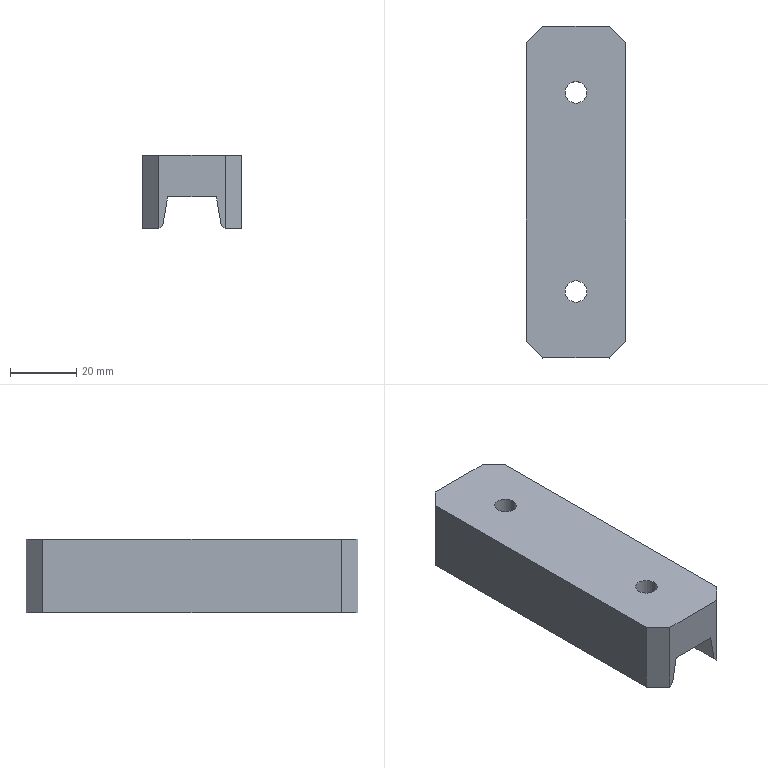Part | Creo | 1 solid | 26 faces | box 30 x 100 x 22 mm | volume 47874 mm3 | plane 18 | cylinder 8 | commonest cylinder face diameters 6.5 x4 10 x4
STEP:
#1=CARTESIAN_POINT('',(-254.325,130.,9.5));
#2=VERTEX_POINT('',#1);
#3=CARTESIAN_POINT('',(-255.826,130.,0.9848));
#4=VERTEX_POINT('',#3);
#5=CARTESIAN_POINT('',(-254.325,130.,9.5));
#6=DIRECTION('',(-0.1736,0.,-0.9848));
#7=VECTOR('',#6,8.647);
#8=LINE('',#5,#7);
#9=EDGE_CURVE('',#2,#4,#8,.T.);
#10=ORIENTED_EDGE('',*,*,#9,.F.);
#11=CARTESIAN_POINT('',(-239.675,130.,9.5));
#12=VERTEX_POINT('',#11);
#13=CARTESIAN_POINT('',(-254.325,130.,9.5));
#14=DIRECTION('',(1.,0.,0.));
#15=VECTOR('',#14,14.65);
#16=LINE('',#13,#15);
#17=EDGE_CURVE('',#2,#12,#16,.T.);
#18=ORIENTED_EDGE('',*,*,#17,.T.);
#19=CARTESIAN_POINT('',(-238.174,130.,0.9848));
#20=VERTEX_POINT('',#19);
#21=CARTESIAN_POINT('',(-238.174,130.,0.9848));
#22=DIRECTION('',(-0.1736,0.,0.9848));
#23=VECTOR('',#22,8.647);
#24=LINE('',#21,#23);
#25=EDGE_CURVE('',#20,#12,#24,.T.);
#26=ORIENTED_EDGE('',*,*,#25,.F.);
#27=CARTESIAN_POINT('',(-237.,130.,0.));
#28=VERTEX_POINT('',#27);
#29=CARTESIAN_POINT('',(-237.,130.,0.));
#30=DIRECTION('',(-0.766,0.,0.6428));
#31=VECTOR('',#30,1.532);
#32=LINE('',#29,#31);
#33=EDGE_CURVE('',#28,#20,#32,.T.);
#34=ORIENTED_EDGE('',*,*,#33,.F.);
#35=CARTESIAN_POINT('',(-237.,130.,22.));
#36=VERTEX_POINT('',#35);
#37=CARTESIAN_POINT('',(-237.,130.,0.));
#38=DIRECTION('',(0.,0.,1.));
#39=VECTOR('',#38,22.);
#40=LINE('',#37,#39);
#41=EDGE_CURVE('',#28,#36,#40,.T.);
#42=ORIENTED_EDGE('',*,*,#41,.T.);
#43=CARTESIAN_POINT('',(-257.,130.,22.));
#44=VERTEX_POINT('',#43);
#45=CARTESIAN_POINT('',(-237.,130.,22.));
#46=DIRECTION('',(-1.,0.,0.));
#47=VECTOR('',#46,20.);
#48=LINE('',#45,#47);
#49=EDGE_CURVE('',#36,#44,#48,.T.);
#50=ORIENTED_EDGE('',*,*,#49,.T.);
#51=CARTESIAN_POINT('',(-257.,130.,0.));
#52=VERTEX_POINT('',#51);
#53=CARTESIAN_POINT('',(-257.,130.,22.));
#54=DIRECTION('',(0.,0.,-1.));
#55=VECTOR('',#54,22.);
#56=LINE('',#53,#55);
#57=EDGE_CURVE('',#44,#52,#56,.T.);
#58=ORIENTED_EDGE('',*,*,#57,.T.);
#59=CARTESIAN_POINT('',(-255.826,130.,0.9848));
#60=DIRECTION('',(-0.766,0.,-0.6428));
#61=VECTOR('',#60,1.532);
#62=LINE('',#59,#61);
#63=EDGE_CURVE('',#4,#52,#62,.T.);
#64=ORIENTED_EDGE('',*,*,#63,.F.);
#65=EDGE_LOOP('',(#10,#18,#26,#34,#42,#50,#58,#64));
#66=FACE_OUTER_BOUND('',#65,.F.);
#67=CARTESIAN_POINT('',(-247.,130.,0.));
#68=DIRECTION('',(0.,1.,0.));
#69=DIRECTION('',(0.,0.,1.));
#70=AXIS2_PLACEMENT_3D('',#67,#68,#69);
#71=PLANE('',#70);
#72=ADVANCED_FACE('',(#66),#71,.T.);
#73=CARTESIAN_POINT('',(-255.826,30.,0.9848));
#74=VERTEX_POINT('',#73);
#75=CARTESIAN_POINT('',(-254.325,30.,9.5));
#76=VERTEX_POINT('',#75);
#77=CARTESIAN_POINT('',(-255.826,30.,0.9848));
#78=DIRECTION('',(0.1736,0.,0.9848));
#79=VECTOR('',#78,8.647);
#80=LINE('',#77,#79);
#81=EDGE_CURVE('',#74,#76,#80,.T.);
#82=ORIENTED_EDGE('',*,*,#81,.T.);
#83=CARTESIAN_POINT('',(-254.325,30.,9.5));
#84=DIRECTION('',(0.,1.,0.));
#85=VECTOR('',#84,100.);
#86=LINE('',#83,#85);
#87=EDGE_CURVE('',#76,#2,#86,.T.);
#88=ORIENTED_EDGE('',*,*,#87,.T.);
#89=ORIENTED_EDGE('',*,*,#9,.T.);
#90=CARTESIAN_POINT('',(-255.826,130.,0.9848));
#91=DIRECTION('',(0.,-1.,0.));
#92=VECTOR('',#91,100.);
#93=LINE('',#90,#92);
#94=EDGE_CURVE('',#4,#74,#93,.T.);
#95=ORIENTED_EDGE('',*,*,#94,.T.);
#96=EDGE_LOOP('',(#82,#88,#89,#95));
#97=FACE_OUTER_BOUND('',#96,.F.);
#98=CARTESIAN_POINT('',(-254.325,130.,9.5));
#99=DIRECTION('',(-0.9848,0.,0.1736));
#100=DIRECTION('',(0.1736,0.,0.9848));
#101=AXIS2_PLACEMENT_3D('',#98,#99,#100);
#102=PLANE('',#101);
#103=ADVANCED_FACE('',(#97),#102,.F.);
#104=CARTESIAN_POINT('',(-257.,30.,0.));
#105=VERTEX_POINT('',#104);
#106=CARTESIAN_POINT('',(-257.,30.,22.));
#107=VERTEX_POINT('',#106);
#108=CARTESIAN_POINT('',(-257.,30.,0.));
#109=DIRECTION('',(0.,0.,1.));
#110=VECTOR('',#109,22.);
#111=LINE('',#108,#110);
#112=EDGE_CURVE('',#105,#107,#111,.T.);
#113=ORIENTED_EDGE('',*,*,#112,.T.);
#114=CARTESIAN_POINT('',(-237.,30.,22.));
#115=VERTEX_POINT('',#114);
#116=CARTESIAN_POINT('',(-257.,30.,22.));
#117=DIRECTION('',(1.,0.,0.));
#118=VECTOR('',#117,20.);
#119=LINE('',#116,#118);
#120=EDGE_CURVE('',#107,#115,#119,.T.);
#121=ORIENTED_EDGE('',*,*,#120,.T.);
#122=CARTESIAN_POINT('',(-237.,30.,0.));
#123=VERTEX_POINT('',#122);
#124=CARTESIAN_POINT('',(-237.,30.,22.));
#125=DIRECTION('',(0.,0.,-1.));
#126=VECTOR('',#125,22.);
#127=LINE('',#124,#126);
#128=EDGE_CURVE('',#115,#123,#127,.T.);
#129=ORIENTED_EDGE('',*,*,#128,.T.);
#130=CARTESIAN_POINT('',(-238.174,30.,0.9848));
#131=VERTEX_POINT('',#130);
#132=CARTESIAN_POINT('',(-238.174,30.,0.9848));
#133=DIRECTION('',(0.766,0.,-0.6428));
#134=VECTOR('',#133,1.532);
#135=LINE('',#132,#134);
#136=EDGE_CURVE('',#131,#123,#135,.T.);
#137=ORIENTED_EDGE('',*,*,#136,.F.);
#138=CARTESIAN_POINT('',(-239.675,30.,9.5));
#139=VERTEX_POINT('',#138);
#140=CARTESIAN_POINT('',(-239.675,30.,9.5));
#141=DIRECTION('',(0.1736,0.,-0.9848));
#142=VECTOR('',#141,8.647);
#143=LINE('',#140,#142);
#144=EDGE_CURVE('',#139,#131,#143,.T.);
#145=ORIENTED_EDGE('',*,*,#144,.F.);
#146=CARTESIAN_POINT('',(-254.325,30.,9.5));
#147=DIRECTION('',(1.,0.,0.));
#148=VECTOR('',#147,14.65);
#149=LINE('',#146,#148);
#150=EDGE_CURVE('',#76,#139,#149,.T.);
#151=ORIENTED_EDGE('',*,*,#150,.F.);
#152=ORIENTED_EDGE('',*,*,#81,.F.);
#153=CARTESIAN_POINT('',(-257.,30.,0.));
#154=DIRECTION('',(0.766,0.,0.6428));
#155=VECTOR('',#154,1.532);
#156=LINE('',#153,#155);
#157=EDGE_CURVE('',#105,#74,#156,.T.);
#158=ORIENTED_EDGE('',*,*,#157,.F.);
#159=EDGE_LOOP('',(#113,#121,#129,#137,#145,#151,#152,#158));
#160=FACE_OUTER_BOUND('',#159,.F.);
#161=CARTESIAN_POINT('',(-247.,30.,0.));
#162=DIRECTION('',(0.,-1.,0.));
#163=DIRECTION('',(0.,0.,-1.));
#164=AXIS2_PLACEMENT_3D('',#161,#162,#163);
#165=PLANE('',#164);
#166=ADVANCED_FACE('',(#160),#165,.T.);
#167=CARTESIAN_POINT('',(-262.,35.,0.));
#168=VERTEX_POINT('',#167);
#169=CARTESIAN_POINT('',(-257.,30.,0.));
#170=DIRECTION('',(-0.7071,0.7071,0.));
#171=VECTOR('',#170,7.071);
#172=LINE('',#169,#171);
#173=EDGE_CURVE('',#105,#168,#172,.T.);
#174=ORIENTED_EDGE('',*,*,#173,.T.);
#175=CARTESIAN_POINT('',(-262.,35.,22.));
#176=VERTEX_POINT('',#175);
#177=CARTESIAN_POINT('',(-262.,35.,22.));
#178=DIRECTION('',(0.,0.,-1.));
#179=VECTOR('',#178,22.);
#180=LINE('',#177,#179);
#181=EDGE_CURVE('',#176,#168,#180,.T.);
#182=ORIENTED_EDGE('',*,*,#181,.F.);
#183=CARTESIAN_POINT('',(-262.,35.,22.));
#184=DIRECTION('',(0.7071,-0.7071,0.));
#185=VECTOR('',#184,7.071);
#186=LINE('',#183,#185);
#187=EDGE_CURVE('',#176,#107,#186,.T.);
#188=ORIENTED_EDGE('',*,*,#187,.T.);
#189=ORIENTED_EDGE('',*,*,#112,.F.);
#190=EDGE_LOOP('',(#174,#182,#188,#189));
#191=FACE_OUTER_BOUND('',#190,.F.);
#192=CARTESIAN_POINT('',(-262.,35.,0.));
#193=DIRECTION('',(0.7071,0.7071,0.));
#194=DIRECTION('',(-0.7071,0.7071,0.));
#195=AXIS2_PLACEMENT_3D('',#192,#193,#194);
#196=PLANE('',#195);
#197=ADVANCED_FACE('',(#191),#196,.F.);
#198=CARTESIAN_POINT('',(-262.,125.,0.));
#199=VERTEX_POINT('',#198);
#200=CARTESIAN_POINT('',(-262.,125.,0.));
#201=DIRECTION('',(0.7071,0.7071,0.));
#202=VECTOR('',#201,7.071);
#203=LINE('',#200,#202);
#204=EDGE_CURVE('',#199,#52,#203,.T.);
#205=ORIENTED_EDGE('',*,*,#204,.F.);
#206=CARTESIAN_POINT('',(-262.,35.,0.));
#207=DIRECTION('',(0.,1.,0.));
#208=VECTOR('',#207,90.);
#209=LINE('',#206,#208);
#210=EDGE_CURVE('',#168,#199,#209,.T.);
#211=ORIENTED_EDGE('',*,*,#210,.F.);
#212=ORIENTED_EDGE('',*,*,#173,.F.);
#213=CARTESIAN_POINT('',(-257.,30.,0.));
#214=DIRECTION('',(0.,1.,0.));
#215=VECTOR('',#214,100.);
#216=LINE('',#213,#215);
#217=EDGE_CURVE('',#105,#52,#216,.T.);
#218=ORIENTED_EDGE('',*,*,#217,.T.);
#219=EDGE_LOOP('',(#205,#211,#212,#218));
#220=FACE_OUTER_BOUND('',#219,.F.);
#221=CARTESIAN_POINT('',(-247.,80.,0.));
#222=DIRECTION('',(0.,0.,-1.));
#223=DIRECTION('',(-1.,0.,0.));
#224=AXIS2_PLACEMENT_3D('',#221,#222,#223);
#225=PLANE('',#224);
#226=ADVANCED_FACE('',(#220),#225,.T.);
#227=ORIENTED_EDGE('',*,*,#204,.T.);
#228=ORIENTED_EDGE('',*,*,#57,.F.);
#229=CARTESIAN_POINT('',(-262.,125.,22.));
#230=VERTEX_POINT('',#229);
#231=CARTESIAN_POINT('',(-257.,130.,22.));
#232=DIRECTION('',(-0.7071,-0.7071,0.));
#233=VECTOR('',#232,7.071);
#234=LINE('',#231,#233);
#235=EDGE_CURVE('',#44,#230,#234,.T.);
#236=ORIENTED_EDGE('',*,*,#235,.T.);
#237=CARTESIAN_POINT('',(-262.,125.,0.));
#238=DIRECTION('',(0.,0.,1.));
#239=VECTOR('',#238,22.);
#240=LINE('',#237,#239);
#241=EDGE_CURVE('',#199,#230,#240,.T.);
#242=ORIENTED_EDGE('',*,*,#241,.F.);
#243=EDGE_LOOP('',(#227,#228,#236,#242));
#244=FACE_OUTER_BOUND('',#243,.F.);
#245=CARTESIAN_POINT('',(-257.,130.,0.));
#246=DIRECTION('',(0.7071,-0.7071,0.));
#247=DIRECTION('',(0.7071,0.7071,0.));
#248=AXIS2_PLACEMENT_3D('',#245,#246,#247);
#249=PLANE('',#248);
#250=ADVANCED_FACE('',(#244),#249,.F.);
#251=ORIENTED_EDGE('',*,*,#49,.F.);
#252=CARTESIAN_POINT('',(-232.,125.,22.));
#253=VERTEX_POINT('',#252);
#254=CARTESIAN_POINT('',(-232.,125.,22.));
#255=DIRECTION('',(-0.7071,0.7071,0.));
#256=VECTOR('',#255,7.071);
#257=LINE('',#254,#256);
#258=EDGE_CURVE('',#253,#36,#257,.T.);
#259=ORIENTED_EDGE('',*,*,#258,.F.);
#260=CARTESIAN_POINT('',(-232.,35.,22.));
#261=VERTEX_POINT('',#260);
#262=CARTESIAN_POINT('',(-232.,35.,22.));
#263=DIRECTION('',(0.,1.,0.));
#264=VECTOR('',#263,90.);
#265=LINE('',#262,#264);
#266=EDGE_CURVE('',#261,#253,#265,.T.);
#267=ORIENTED_EDGE('',*,*,#266,.F.);
#268=CARTESIAN_POINT('',(-237.,30.,22.));
#269=DIRECTION('',(0.7071,0.7071,0.));
#270=VECTOR('',#269,7.071);
#271=LINE('',#268,#270);
#272=EDGE_CURVE('',#115,#261,#271,.T.);
#273=ORIENTED_EDGE('',*,*,#272,.F.);
#274=ORIENTED_EDGE('',*,*,#120,.F.);
#275=ORIENTED_EDGE('',*,*,#187,.F.);
#276=CARTESIAN_POINT('',(-262.,125.,22.));
#277=DIRECTION('',(0.,-1.,0.));
#278=VECTOR('',#277,90.);
#279=LINE('',#276,#278);
#280=EDGE_CURVE('',#230,#176,#279,.T.);
#281=ORIENTED_EDGE('',*,*,#280,.F.);
#282=ORIENTED_EDGE('',*,*,#235,.F.);
#283=EDGE_LOOP('',(#251,#259,#267,#273,#274,#275,#281,#282));
#284=FACE_OUTER_BOUND('',#283,.F.);
#285=CARTESIAN_POINT('',(-243.75,110.,22.));
#286=VERTEX_POINT('',#285);
#287=CARTESIAN_POINT('',(-250.25,110.,22.));
#288=VERTEX_POINT('',#287);
#289=CARTESIAN_POINT('',(-247.,110.,22.));
#290=DIRECTION('',(0.,0.,-1.));
#291=DIRECTION('',(1.,0.,0.));
#292=AXIS2_PLACEMENT_3D('',#289,#290,#291);
#293=CIRCLE('',#292,3.25);
#294=EDGE_CURVE('',#286,#288,#293,.T.);
#295=ORIENTED_EDGE('',*,*,#294,.F.);
#296=CARTESIAN_POINT('',(-247.,110.,22.));
#297=DIRECTION('',(0.,0.,-1.));
#298=DIRECTION('',(-1.,0.,0.));
#299=AXIS2_PLACEMENT_3D('',#296,#297,#298);
#300=CIRCLE('',#299,3.25);
#301=EDGE_CURVE('',#288,#286,#300,.T.);
#302=ORIENTED_EDGE('',*,*,#301,.F.);
#303=EDGE_LOOP('',(#295,#302));
#304=FACE_BOUND('',#303,.F.);
#305=CARTESIAN_POINT('',(-243.75,50.,22.));
#306=VERTEX_POINT('',#305);
#307=CARTESIAN_POINT('',(-250.25,50.,22.));
#308=VERTEX_POINT('',#307);
#309=CARTESIAN_POINT('',(-247.,50.,22.));
#310=DIRECTION('',(0.,0.,-1.));
#311=DIRECTION('',(1.,0.,0.));
#312=AXIS2_PLACEMENT_3D('',#309,#310,#311);
#313=CIRCLE('',#312,3.25);
#314=EDGE_CURVE('',#306,#308,#313,.T.);
#315=ORIENTED_EDGE('',*,*,#314,.F.);
#316=CARTESIAN_POINT('',(-247.,50.,22.));
#317=DIRECTION('',(0.,0.,-1.));
#318=DIRECTION('',(-1.,0.,0.));
#319=AXIS2_PLACEMENT_3D('',#316,#317,#318);
#320=CIRCLE('',#319,3.25);
#321=EDGE_CURVE('',#308,#306,#320,.T.);
#322=ORIENTED_EDGE('',*,*,#321,.F.);
#323=EDGE_LOOP('',(#315,#322));
#324=FACE_BOUND('',#323,.F.);
#325=CARTESIAN_POINT('',(-247.,80.,22.));
#326=DIRECTION('',(0.,0.,1.));
#327=DIRECTION('',(1.,0.,0.));
#328=AXIS2_PLACEMENT_3D('',#325,#326,#327);
#329=PLANE('',#328);
#330=ADVANCED_FACE('',(#284,#304,#324),#329,.T.);
#331=CARTESIAN_POINT('',(-250.25,50.,16.));
#332=VERTEX_POINT('',#331);
#333=CARTESIAN_POINT('',(-243.75,50.,16.));
#334=VERTEX_POINT('',#333);
#335=CARTESIAN_POINT('',(-247.,50.,16.));
#336=DIRECTION('',(0.,0.,1.));
#337=DIRECTION('',(-1.,0.,0.));
#338=AXIS2_PLACEMENT_3D('',#335,#336,#337);
#339=CIRCLE('',#338,3.25);
#340=EDGE_CURVE('',#332,#334,#339,.T.);
#341=ORIENTED_EDGE('',*,*,#340,.T.);
#342=CARTESIAN_POINT('',(-243.75,50.,16.));
#343=DIRECTION('',(0.,0.,1.));
#344=VECTOR('',#343,6.);
#345=LINE('',#342,#344);
#346=EDGE_CURVE('',#334,#306,#345,.T.);
#347=ORIENTED_EDGE('',*,*,#346,.T.);
#348=ORIENTED_EDGE('',*,*,#314,.T.);
#349=CARTESIAN_POINT('',(-250.25,50.,16.));
#350=DIRECTION('',(0.,0.,1.));
#351=VECTOR('',#350,6.);
#352=LINE('',#349,#351);
#353=EDGE_CURVE('',#332,#308,#352,.T.);
#354=ORIENTED_EDGE('',*,*,#353,.F.);
#355=EDGE_LOOP('',(#341,#347,#348,#354));
#356=FACE_OUTER_BOUND('',#355,.F.);
#357=CARTESIAN_POINT('',(-247.,50.,9.5));
#358=DIRECTION('',(0.,0.,1.));
#359=DIRECTION('',(1.,0.,0.));
#360=AXIS2_PLACEMENT_3D('',#357,#358,#359);
#361=CYLINDRICAL_SURFACE('',#360,3.25);
#362=ADVANCED_FACE('',(#356),#361,.F.);
#363=CARTESIAN_POINT('',(-252.,50.,16.));
#364=VERTEX_POINT('',#363);
#365=CARTESIAN_POINT('',(-242.,50.,16.));
#366=VERTEX_POINT('',#365);
#367=CARTESIAN_POINT('',(-247.,50.,16.));
#368=DIRECTION('',(0.,0.,-1.));
#369=DIRECTION('',(-1.,0.,0.));
#370=AXIS2_PLACEMENT_3D('',#367,#368,#369);
#371=CIRCLE('',#370,5.);
#372=EDGE_CURVE('',#364,#366,#371,.T.);
#373=ORIENTED_EDGE('',*,*,#372,.F.);
#374=CARTESIAN_POINT('',(-247.,50.,16.));
#375=DIRECTION('',(0.,0.,-1.));
#376=DIRECTION('',(1.,0.,0.));
#377=AXIS2_PLACEMENT_3D('',#374,#375,#376);
#378=CIRCLE('',#377,5.);
#379=EDGE_CURVE('',#366,#364,#378,.T.);
#380=ORIENTED_EDGE('',*,*,#379,.F.);
#381=EDGE_LOOP('',(#373,#380));
#382=FACE_OUTER_BOUND('',#381,.F.);
#383=CARTESIAN_POINT('',(-247.,50.,16.));
#384=DIRECTION('',(0.,0.,1.));
#385=DIRECTION('',(1.,0.,0.));
#386=AXIS2_PLACEMENT_3D('',#383,#384,#385);
#387=CIRCLE('',#386,3.25);
#388=EDGE_CURVE('',#334,#332,#387,.T.);
#389=ORIENTED_EDGE('',*,*,#388,.F.);
#390=ORIENTED_EDGE('',*,*,#340,.F.);
#391=EDGE_LOOP('',(#389,#390));
#392=FACE_BOUND('',#391,.F.);
#393=CARTESIAN_POINT('',(-247.,50.,16.));
#394=DIRECTION('',(0.,0.,1.));
#395=DIRECTION('',(1.,0.,0.));
#396=AXIS2_PLACEMENT_3D('',#393,#394,#395);
#397=PLANE('',#396);
#398=ADVANCED_FACE('',(#382,#392),#397,.F.);
#399=ORIENTED_EDGE('',*,*,#372,.T.);
#400=CARTESIAN_POINT('',(-242.,50.,9.5));
#401=VERTEX_POINT('',#400);
#402=CARTESIAN_POINT('',(-242.,50.,9.5));
#403=DIRECTION('',(0.,0.,1.));
#404=VECTOR('',#403,6.5);
#405=LINE('',#402,#404);
#406=EDGE_CURVE('',#401,#366,#405,.T.);
#407=ORIENTED_EDGE('',*,*,#406,.F.);
#408=CARTESIAN_POINT('',(-252.,50.,9.5));
#409=VERTEX_POINT('',#408);
#410=CARTESIAN_POINT('',(-247.,50.,9.5));
#411=DIRECTION('',(0.,0.,1.));
#412=DIRECTION('',(1.,0.,0.));
#413=AXIS2_PLACEMENT_3D('',#410,#411,#412);
#414=CIRCLE('',#413,5.);
#415=EDGE_CURVE('',#401,#409,#414,.T.);
#416=ORIENTED_EDGE('',*,*,#415,.T.);
#417=CARTESIAN_POINT('',(-252.,50.,9.5));
#418=DIRECTION('',(0.,0.,1.));
#419=VECTOR('',#418,6.5);
#420=LINE('',#417,#419);
#421=EDGE_CURVE('',#409,#364,#420,.T.);
#422=ORIENTED_EDGE('',*,*,#421,.T.);
#423=EDGE_LOOP('',(#399,#407,#416,#422));
#424=FACE_OUTER_BOUND('',#423,.F.);
#425=CARTESIAN_POINT('',(-247.,50.,9.5));
#426=DIRECTION('',(0.,0.,1.));
#427=DIRECTION('',(1.,0.,0.));
#428=AXIS2_PLACEMENT_3D('',#425,#426,#427);
#429=CYLINDRICAL_SURFACE('',#428,5.);
#430=ADVANCED_FACE('',(#424),#429,.F.);
#431=ORIENTED_EDGE('',*,*,#379,.T.);
#432=ORIENTED_EDGE('',*,*,#421,.F.);
#433=CARTESIAN_POINT('',(-247.,50.,9.5));
#434=DIRECTION('',(0.,0.,1.));
#435=DIRECTION('',(-1.,0.,0.));
#436=AXIS2_PLACEMENT_3D('',#433,#434,#435);
#437=CIRCLE('',#436,5.);
#438=EDGE_CURVE('',#409,#401,#437,.T.);
#439=ORIENTED_EDGE('',*,*,#438,.T.);
#440=ORIENTED_EDGE('',*,*,#406,.T.);
#441=EDGE_LOOP('',(#431,#432,#439,#440));
#442=FACE_OUTER_BOUND('',#441,.F.);
#443=CARTESIAN_POINT('',(-247.,50.,9.5));
#444=DIRECTION('',(0.,0.,1.));
#445=DIRECTION('',(1.,0.,0.));
#446=AXIS2_PLACEMENT_3D('',#443,#444,#445);
#447=CYLINDRICAL_SURFACE('',#446,5.);
#448=ADVANCED_FACE('',(#442),#447,.F.);
#449=ORIENTED_EDGE('',*,*,#150,.T.);
#450=CARTESIAN_POINT('',(-239.675,30.,9.5));
#451=DIRECTION('',(0.,1.,0.));
#452=VECTOR('',#451,100.);
#453=LINE('',#450,#452);
#454=EDGE_CURVE('',#139,#12,#453,.T.);
#455=ORIENTED_EDGE('',*,*,#454,.T.);
#456=ORIENTED_EDGE('',*,*,#17,.F.);
#457=ORIENTED_EDGE('',*,*,#87,.F.);
#458=EDGE_LOOP('',(#449,#455,#456,#457));
#459=FACE_OUTER_BOUND('',#458,.F.);
#460=CARTESIAN_POINT('',(-242.,110.,9.5));
#461=VERTEX_POINT('',#460);
#462=CARTESIAN_POINT('',(-252.,110.,9.5));
#463=VERTEX_POINT('',#462);
#464=CARTESIAN_POINT('',(-247.,110.,9.5));
#465=DIRECTION('',(0.,0.,1.));
#466=DIRECTION('',(1.,0.,0.));
#467=AXIS2_PLACEMENT_3D('',#464,#465,#466);
#468=CIRCLE('',#467,5.);
#469=EDGE_CURVE('',#461,#463,#468,.T.);
#470=ORIENTED_EDGE('',*,*,#469,.F.);
#471=CARTESIAN_POINT('',(-247.,110.,9.5));
#472=DIRECTION('',(0.,0.,1.));
#473=DIRECTION('',(-1.,0.,0.));
#474=AXIS2_PLACEMENT_3D('',#471,#472,#473);
#475=CIRCLE('',#474,5.);
#476=EDGE_CURVE('',#463,#461,#475,.T.);
#477=ORIENTED_EDGE('',*,*,#476,.F.);
#478=EDGE_LOOP('',(#470,#477));
#479=FACE_BOUND('',#478,.F.);
#480=ORIENTED_EDGE('',*,*,#415,.F.);
#481=ORIENTED_EDGE('',*,*,#438,.F.);
#482=EDGE_LOOP('',(#480,#481));
#483=FACE_BOUND('',#482,.F.);
#484=CARTESIAN_POINT('',(-239.675,130.,9.5));
#485=DIRECTION('',(0.,0.,1.));
#486=DIRECTION('',(1.,0.,0.));
#487=AXIS2_PLACEMENT_3D('',#484,#485,#486);
#488=PLANE('',#487);
#489=ADVANCED_FACE('',(#459,#479,#483),#488,.F.);
#490=CARTESIAN_POINT('',(-252.,110.,16.));
#491=VERTEX_POINT('',#490);
#492=CARTESIAN_POINT('',(-242.,110.,16.));
#493=VERTEX_POINT('',#492);
#494=CARTESIAN_POINT('',(-247.,110.,16.));
#495=DIRECTION('',(0.,0.,-1.));
#496=DIRECTION('',(-1.,0.,0.));
#497=AXIS2_PLACEMENT_3D('',#494,#495,#496);
#498=CIRCLE('',#497,5.);
#499=EDGE_CURVE('',#491,#493,#498,.T.);
#500=ORIENTED_EDGE('',*,*,#499,.T.);
#501=CARTESIAN_POINT('',(-242.,110.,9.5));
#502=DIRECTION('',(0.,0.,1.));
#503=VECTOR('',#502,6.5);
#504=LINE('',#501,#503);
#505=EDGE_CURVE('',#461,#493,#504,.T.);
#506=ORIENTED_EDGE('',*,*,#505,.F.);
#507=ORIENTED_EDGE('',*,*,#469,.T.);
#508=CARTESIAN_POINT('',(-252.,110.,9.5));
#509=DIRECTION('',(0.,0.,1.));
#510=VECTOR('',#509,6.5);
#511=LINE('',#508,#510);
#512=EDGE_CURVE('',#463,#491,#511,.T.);
#513=ORIENTED_EDGE('',*,*,#512,.T.);
#514=EDGE_LOOP('',(#500,#506,#507,#513));
#515=FACE_OUTER_BOUND('',#514,.F.);
#516=CARTESIAN_POINT('',(-247.,110.,9.5));
#517=DIRECTION('',(0.,0.,1.));
#518=DIRECTION('',(1.,0.,0.));
#519=AXIS2_PLACEMENT_3D('',#516,#517,#518);
#520=CYLINDRICAL_SURFACE('',#519,5.);
#521=ADVANCED_FACE('',(#515),#520,.F.);
#522=ORIENTED_EDGE('',*,*,#499,.F.);
#523=CARTESIAN_POINT('',(-247.,110.,16.));
#524=DIRECTION('',(0.,0.,-1.));
#525=DIRECTION('',(1.,0.,0.));
#526=AXIS2_PLACEMENT_3D('',#523,#524,#525);
#527=CIRCLE('',#526,5.);
#528=EDGE_CURVE('',#493,#491,#527,.T.);
#529=ORIENTED_EDGE('',*,*,#528,.F.);
#530=EDGE_LOOP('',(#522,#529));
#531=FACE_OUTER_BOUND('',#530,.F.);
#532=CARTESIAN_POINT('',(-243.75,110.,16.));
#533=VERTEX_POINT('',#532);
#534=CARTESIAN_POINT('',(-250.25,110.,16.));
#535=VERTEX_POINT('',#534);
#536=CARTESIAN_POINT('',(-247.,110.,16.));
#537=DIRECTION('',(0.,0.,1.));
#538=DIRECTION('',(1.,0.,0.));
#539=AXIS2_PLACEMENT_3D('',#536,#537,#538);
#540=CIRCLE('',#539,3.25);
#541=EDGE_CURVE('',#533,#535,#540,.T.);
#542=ORIENTED_EDGE('',*,*,#541,.F.);
#543=CARTESIAN_POINT('',(-247.,110.,16.));
#544=DIRECTION('',(0.,0.,1.));
#545=DIRECTION('',(-1.,0.,0.));
#546=AXIS2_PLACEMENT_3D('',#543,#544,#545);
#547=CIRCLE('',#546,3.25);
#548=EDGE_CURVE('',#535,#533,#547,.T.);
#549=ORIENTED_EDGE('',*,*,#548,.F.);
#550=EDGE_LOOP('',(#542,#549));
#551=FACE_BOUND('',#550,.F.);
#552=CARTESIAN_POINT('',(-247.,110.,16.));
#553=DIRECTION('',(0.,0.,1.));
#554=DIRECTION('',(1.,0.,0.));
#555=AXIS2_PLACEMENT_3D('',#552,#553,#554);
#556=PLANE('',#555);
#557=ADVANCED_FACE('',(#531,#551),#556,.F.);
#558=ORIENTED_EDGE('',*,*,#528,.T.);
#559=ORIENTED_EDGE('',*,*,#512,.F.);
#560=ORIENTED_EDGE('',*,*,#476,.T.);
#561=ORIENTED_EDGE('',*,*,#505,.T.);
#562=EDGE_LOOP('',(#558,#559,#560,#561));
#563=FACE_OUTER_BOUND('',#562,.F.);
#564=CARTESIAN_POINT('',(-247.,110.,9.5));
#565=DIRECTION('',(0.,0.,1.));
#566=DIRECTION('',(1.,0.,0.));
#567=AXIS2_PLACEMENT_3D('',#564,#565,#566);
#568=CYLINDRICAL_SURFACE('',#567,5.);
#569=ADVANCED_FACE('',(#563),#568,.F.);
#570=ORIENTED_EDGE('',*,*,#541,.T.);
#571=CARTESIAN_POINT('',(-250.25,110.,16.));
#572=DIRECTION('',(0.,0.,1.));
#573=VECTOR('',#572,6.);
#574=LINE('',#571,#573);
#575=EDGE_CURVE('',#535,#288,#574,.T.);
#576=ORIENTED_EDGE('',*,*,#575,.T.);
#577=ORIENTED_EDGE('',*,*,#301,.T.);
#578=CARTESIAN_POINT('',(-243.75,110.,16.));
#579=DIRECTION('',(0.,0.,1.));
#580=VECTOR('',#579,6.);
#581=LINE('',#578,#580);
#582=EDGE_CURVE('',#533,#286,#581,.T.);
#583=ORIENTED_EDGE('',*,*,#582,.F.);
#584=EDGE_LOOP('',(#570,#576,#577,#583));
#585=FACE_OUTER_BOUND('',#584,.F.);
#586=CARTESIAN_POINT('',(-247.,110.,9.5));
#587=DIRECTION('',(0.,0.,1.));
#588=DIRECTION('',(1.,0.,0.));
#589=AXIS2_PLACEMENT_3D('',#586,#587,#588);
#590=CYLINDRICAL_SURFACE('',#589,3.25);
#591=ADVANCED_FACE('',(#585),#590,.F.);
#592=ORIENTED_EDGE('',*,*,#548,.T.);
#593=ORIENTED_EDGE('',*,*,#582,.T.);
#594=ORIENTED_EDGE('',*,*,#294,.T.);
#595=ORIENTED_EDGE('',*,*,#575,.F.);
#596=EDGE_LOOP('',(#592,#593,#594,#595));
#597=FACE_OUTER_BOUND('',#596,.F.);
#598=CARTESIAN_POINT('',(-247.,110.,9.5));
#599=DIRECTION('',(0.,0.,1.));
#600=DIRECTION('',(1.,0.,0.));
#601=AXIS2_PLACEMENT_3D('',#598,#599,#600);
#602=CYLINDRICAL_SURFACE('',#601,3.25);
#603=ADVANCED_FACE('',(#597),#602,.F.);
#604=ORIENTED_EDGE('',*,*,#25,.T.);
#605=ORIENTED_EDGE('',*,*,#454,.F.);
#606=ORIENTED_EDGE('',*,*,#144,.T.);
#607=CARTESIAN_POINT('',(-238.174,30.,0.9848));
#608=DIRECTION('',(0.,1.,0.));
#609=VECTOR('',#608,100.);
#610=LINE('',#607,#609);
#611=EDGE_CURVE('',#131,#20,#610,.T.);
#612=ORIENTED_EDGE('',*,*,#611,.T.);
#613=EDGE_LOOP('',(#604,#605,#606,#612));
#614=FACE_OUTER_BOUND('',#613,.F.);
#615=CARTESIAN_POINT('',(-238.,130.,0.));
#616=DIRECTION('',(0.9848,0.,0.1736));
#617=DIRECTION('',(0.1736,0.,-0.9848));
#618=AXIS2_PLACEMENT_3D('',#615,#616,#617);
#619=PLANE('',#618);
#620=ADVANCED_FACE('',(#614),#619,.F.);
#621=ORIENTED_EDGE('',*,*,#33,.T.);
#622=ORIENTED_EDGE('',*,*,#611,.F.);
#623=ORIENTED_EDGE('',*,*,#136,.T.);
#624=CARTESIAN_POINT('',(-237.,130.,0.));
#625=DIRECTION('',(0.,-1.,0.));
#626=VECTOR('',#625,100.);
#627=LINE('',#624,#626);
#628=EDGE_CURVE('',#28,#123,#627,.T.);
#629=ORIENTED_EDGE('',*,*,#628,.F.);
#630=EDGE_LOOP('',(#621,#622,#623,#629));
#631=FACE_OUTER_BOUND('',#630,.F.);
#632=CARTESIAN_POINT('',(-238.174,130.,0.9848));
#633=DIRECTION('',(-0.6428,0.,-0.766));
#634=DIRECTION('',(-0.766,0.,0.6428));
#635=AXIS2_PLACEMENT_3D('',#632,#633,#634);
#636=PLANE('',#635);
#637=ADVANCED_FACE('',(#631),#636,.T.);
#638=CARTESIAN_POINT('',(-232.,35.,0.));
#639=VERTEX_POINT('',#638);
#640=CARTESIAN_POINT('',(-232.,35.,0.));
#641=DIRECTION('',(-0.7071,-0.7071,0.));
#642=VECTOR('',#641,7.071);
#643=LINE('',#640,#642);
#644=EDGE_CURVE('',#639,#123,#643,.T.);
#645=ORIENTED_EDGE('',*,*,#644,.F.);
#646=CARTESIAN_POINT('',(-232.,125.,0.));
#647=VERTEX_POINT('',#646);
#648=CARTESIAN_POINT('',(-232.,125.,0.));
#649=DIRECTION('',(0.,-1.,0.));
#650=VECTOR('',#649,90.);
#651=LINE('',#648,#650);
#652=EDGE_CURVE('',#647,#639,#651,.T.);
#653=ORIENTED_EDGE('',*,*,#652,.F.);
#654=CARTESIAN_POINT('',(-237.,130.,0.));
#655=DIRECTION('',(0.7071,-0.7071,0.));
#656=VECTOR('',#655,7.071);
#657=LINE('',#654,#656);
#658=EDGE_CURVE('',#28,#647,#657,.T.);
#659=ORIENTED_EDGE('',*,*,#658,.F.);
#660=ORIENTED_EDGE('',*,*,#628,.T.);
#661=EDGE_LOOP('',(#645,#653,#659,#660));
#662=FACE_OUTER_BOUND('',#661,.F.);
#663=CARTESIAN_POINT('',(-247.,80.,0.));
#664=DIRECTION('',(0.,0.,-1.));
#665=DIRECTION('',(-1.,0.,0.));
#666=AXIS2_PLACEMENT_3D('',#663,#664,#665);
#667=PLANE('',#666);
#668=ADVANCED_FACE('',(#662),#667,.T.);
#669=ORIENTED_EDGE('',*,*,#644,.T.);
#670=ORIENTED_EDGE('',*,*,#128,.F.);
#671=ORIENTED_EDGE('',*,*,#272,.T.);
#672=CARTESIAN_POINT('',(-232.,35.,0.));
#673=DIRECTION('',(0.,0.,1.));
#674=VECTOR('',#673,22.);
#675=LINE('',#672,#674);
#676=EDGE_CURVE('',#639,#261,#675,.T.);
#677=ORIENTED_EDGE('',*,*,#676,.F.);
#678=EDGE_LOOP('',(#669,#670,#671,#677));
#679=FACE_OUTER_BOUND('',#678,.F.);
#680=CARTESIAN_POINT('',(-237.,30.,0.));
#681=DIRECTION('',(-0.7071,0.7071,0.));
#682=DIRECTION('',(-0.7071,-0.7071,0.));
#683=AXIS2_PLACEMENT_3D('',#680,#681,#682);
#684=PLANE('',#683);
#685=ADVANCED_FACE('',(#679),#684,.F.);
#686=ORIENTED_EDGE('',*,*,#652,.T.);
#687=ORIENTED_EDGE('',*,*,#676,.T.);
#688=ORIENTED_EDGE('',*,*,#266,.T.);
#689=CARTESIAN_POINT('',(-232.,125.,22.));
#690=DIRECTION('',(0.,0.,-1.));
#691=VECTOR('',#690,22.);
#692=LINE('',#689,#691);
#693=EDGE_CURVE('',#253,#647,#692,.T.);
#694=ORIENTED_EDGE('',*,*,#693,.T.);
#695=EDGE_LOOP('',(#686,#687,#688,#694));
#696=FACE_OUTER_BOUND('',#695,.F.);
#697=CARTESIAN_POINT('',(-232.,80.,0.));
#698=DIRECTION('',(1.,0.,0.));
#699=DIRECTION('',(0.,0.,-1.));
#700=AXIS2_PLACEMENT_3D('',#697,#698,#699);
#701=PLANE('',#700);
#702=ADVANCED_FACE('',(#696),#701,.T.);
#703=ORIENTED_EDGE('',*,*,#658,.T.);
#704=ORIENTED_EDGE('',*,*,#693,.F.);
#705=ORIENTED_EDGE('',*,*,#258,.T.);
#706=ORIENTED_EDGE('',*,*,#41,.F.);
#707=EDGE_LOOP('',(#703,#704,#705,#706));
#708=FACE_OUTER_BOUND('',#707,.F.);
#709=CARTESIAN_POINT('',(-232.,125.,0.));
#710=DIRECTION('',(-0.7071,-0.7071,0.));
#711=DIRECTION('',(0.7071,-0.7071,0.));
#712=AXIS2_PLACEMENT_3D('',#709,#710,#711);
#713=PLANE('',#712);
#714=ADVANCED_FACE('',(#708),#713,.F.);
#715=ORIENTED_EDGE('',*,*,#388,.T.);
#716=ORIENTED_EDGE('',*,*,#353,.T.);
#717=ORIENTED_EDGE('',*,*,#321,.T.);
#718=ORIENTED_EDGE('',*,*,#346,.F.);
#719=EDGE_LOOP('',(#715,#716,#717,#718));
#720=FACE_OUTER_BOUND('',#719,.F.);
#721=CARTESIAN_POINT('',(-247.,50.,9.5));
#722=DIRECTION('',(0.,0.,1.));
#723=DIRECTION('',(1.,0.,0.));
#724=AXIS2_PLACEMENT_3D('',#721,#722,#723);
#725=CYLINDRICAL_SURFACE('',#724,3.25);
#726=ADVANCED_FACE('',(#720),#725,.F.);
#727=ORIENTED_EDGE('',*,*,#280,.T.);
#728=ORIENTED_EDGE('',*,*,#181,.T.);
#729=ORIENTED_EDGE('',*,*,#210,.T.);
#730=ORIENTED_EDGE('',*,*,#241,.T.);
#731=EDGE_LOOP('',(#727,#728,#729,#730));
#732=FACE_OUTER_BOUND('',#731,.F.);
#733=CARTESIAN_POINT('',(-262.,80.,0.));
#734=DIRECTION('',(-1.,0.,0.));
#735=DIRECTION('',(0.,0.,1.));
#736=AXIS2_PLACEMENT_3D('',#733,#734,#735);
#737=PLANE('',#736);
#738=ADVANCED_FACE('',(#732),#737,.T.);
#739=ORIENTED_EDGE('',*,*,#63,.T.);
#740=ORIENTED_EDGE('',*,*,#217,.F.);
#741=ORIENTED_EDGE('',*,*,#157,.T.);
#742=ORIENTED_EDGE('',*,*,#94,.F.);
#743=EDGE_LOOP('',(#739,#740,#741,#742));
#744=FACE_OUTER_BOUND('',#743,.F.);
#745=CARTESIAN_POINT('',(-257.,80.,0.));
#746=DIRECTION('',(0.6428,0.,-0.766));
#747=DIRECTION('',(-0.766,0.,-0.6428));
#748=AXIS2_PLACEMENT_3D('',#745,#746,#747);
#749=PLANE('',#748);
#750=ADVANCED_FACE('',(#744),#749,.T.);
#751=CLOSED_SHELL('',(#72,#103,#166,#197,#226,#250,#330,#362,#398,#430,#448,#489,#521,#557,#569,#591,#603,#620,#637,#668,#685,#702,#714,#726,#738,#750));
#752=MANIFOLD_SOLID_BREP('',#751);
#753=(LENGTH_UNIT()NAMED_UNIT(*)SI_UNIT(.MILLI.,.METRE.));
#754=UNCERTAINTY_MEASURE_WITH_UNIT(LENGTH_MEASURE(0.01067),#753,'','');
#755=(NAMED_UNIT(*)PLANE_ANGLE_UNIT()SI_UNIT($,.RADIAN.));
#756=PLANE_ANGLE_MEASURE_WITH_UNIT(PLANE_ANGLE_MEASURE(0.01745),#755);
#757=(CONVERSION_BASED_UNIT('DEGREE',#756)NAMED_UNIT(*)PLANE_ANGLE_UNIT());
#758=(NAMED_UNIT(*)SI_UNIT($,.STERADIAN.)SOLID_ANGLE_UNIT());
#759=(GEOMETRIC_REPRESENTATION_CONTEXT(3)GLOBAL_UNCERTAINTY_ASSIGNED_CONTEXT((#754))GLOBAL_UNIT_ASSIGNED_CONTEXT((#753,#757,#758))REPRESENTATION_CONTEXT('',''));
#760=ADVANCED_BREP_SHAPE_REPRESENTATION('',(#752),#759);